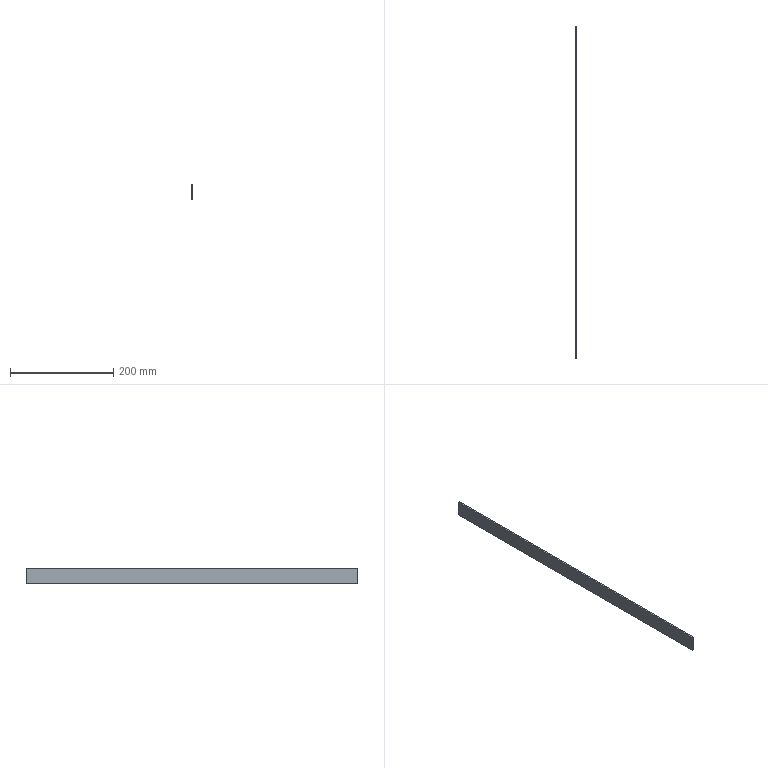Part | SolidWorks | 1 solid | 6 faces | box 3 x 642 x 30 mm | volume 57780 mm3 | plane 6
STEP:
#1=CARTESIAN_POINT('',(0.,321.,15.));
#2=VERTEX_POINT('',#1);
#3=CARTESIAN_POINT('',(0.,-321.,15.));
#4=VERTEX_POINT('',#3);
#5=CARTESIAN_POINT('',(0.,-321.,15.));
#6=DIRECTION('',(0.,-1.,0.));
#7=VECTOR('',#6,1000.);
#8=LINE('',#5,#7);
#9=EDGE_CURVE('',#2,#4,#8,.T.);
#10=ORIENTED_EDGE('',*,*,#9,.F.);
#11=CARTESIAN_POINT('',(-3.,321.,15.));
#12=VERTEX_POINT('',#11);
#13=CARTESIAN_POINT('',(-3.,321.,15.));
#14=DIRECTION('',(1.,0.,0.));
#15=VECTOR('',#14,1000.);
#16=LINE('',#13,#15);
#17=EDGE_CURVE('',#12,#2,#16,.T.);
#18=ORIENTED_EDGE('',*,*,#17,.F.);
#19=CARTESIAN_POINT('',(-3.,-321.,15.));
#20=VERTEX_POINT('',#19);
#21=CARTESIAN_POINT('',(-3.,-321.,15.));
#22=DIRECTION('',(0.,-1.,0.));
#23=VECTOR('',#22,1000.);
#24=LINE('',#21,#23);
#25=EDGE_CURVE('',#12,#20,#24,.T.);
#26=ORIENTED_EDGE('',*,*,#25,.T.);
#27=CARTESIAN_POINT('',(-3.,-321.,15.));
#28=DIRECTION('',(1.,0.,0.));
#29=VECTOR('',#28,1000.);
#30=LINE('',#27,#29);
#31=EDGE_CURVE('',#20,#4,#30,.T.);
#32=ORIENTED_EDGE('',*,*,#31,.T.);
#33=EDGE_LOOP('',(#10,#18,#26,#32));
#34=FACE_OUTER_BOUND('',#33,.T.);
#35=CARTESIAN_POINT('',(-3.,-321.,15.));
#36=DIRECTION('',(0.,0.,1.));
#37=DIRECTION('',(1.,0.,0.));
#38=AXIS2_PLACEMENT_3D('',#35,#36,#37);
#39=PLANE('',#38);
#40=ADVANCED_FACE('',(#34),#39,.T.);
#41=CARTESIAN_POINT('',(0.,321.,-15.));
#42=VERTEX_POINT('',#41);
#43=CARTESIAN_POINT('',(0.,321.,-15.));
#44=DIRECTION('',(0.,0.,1.));
#45=VECTOR('',#44,1000.);
#46=LINE('',#43,#45);
#47=EDGE_CURVE('',#42,#2,#46,.T.);
#48=ORIENTED_EDGE('',*,*,#47,.F.);
#49=CARTESIAN_POINT('',(-3.,321.,-15.));
#50=VERTEX_POINT('',#49);
#51=CARTESIAN_POINT('',(-3.,321.,-15.));
#52=DIRECTION('',(1.,0.,0.));
#53=VECTOR('',#52,1000.);
#54=LINE('',#51,#53);
#55=EDGE_CURVE('',#50,#42,#54,.T.);
#56=ORIENTED_EDGE('',*,*,#55,.F.);
#57=CARTESIAN_POINT('',(-3.,321.,-15.));
#58=DIRECTION('',(0.,0.,1.));
#59=VECTOR('',#58,1000.);
#60=LINE('',#57,#59);
#61=EDGE_CURVE('',#50,#12,#60,.T.);
#62=ORIENTED_EDGE('',*,*,#61,.T.);
#63=ORIENTED_EDGE('',*,*,#17,.T.);
#64=EDGE_LOOP('',(#48,#56,#62,#63));
#65=FACE_OUTER_BOUND('',#64,.T.);
#66=CARTESIAN_POINT('',(-3.,321.,-15.));
#67=DIRECTION('',(0.,1.,0.));
#68=DIRECTION('',(0.,0.,1.));
#69=AXIS2_PLACEMENT_3D('',#66,#67,#68);
#70=PLANE('',#69);
#71=ADVANCED_FACE('',(#65),#70,.T.);
#72=CARTESIAN_POINT('',(0.,-321.,-15.));
#73=VERTEX_POINT('',#72);
#74=CARTESIAN_POINT('',(0.,-321.,-15.));
#75=DIRECTION('',(0.,1.,0.));
#76=VECTOR('',#75,1000.);
#77=LINE('',#74,#76);
#78=EDGE_CURVE('',#73,#42,#77,.T.);
#79=ORIENTED_EDGE('',*,*,#78,.F.);
#80=CARTESIAN_POINT('',(-3.,-321.,-15.));
#81=VERTEX_POINT('',#80);
#82=CARTESIAN_POINT('',(-3.,-321.,-15.));
#83=DIRECTION('',(1.,0.,0.));
#84=VECTOR('',#83,1000.);
#85=LINE('',#82,#84);
#86=EDGE_CURVE('',#81,#73,#85,.T.);
#87=ORIENTED_EDGE('',*,*,#86,.F.);
#88=CARTESIAN_POINT('',(-3.,-321.,-15.));
#89=DIRECTION('',(0.,1.,0.));
#90=VECTOR('',#89,1000.);
#91=LINE('',#88,#90);
#92=EDGE_CURVE('',#81,#50,#91,.T.);
#93=ORIENTED_EDGE('',*,*,#92,.T.);
#94=ORIENTED_EDGE('',*,*,#55,.T.);
#95=EDGE_LOOP('',(#79,#87,#93,#94));
#96=FACE_OUTER_BOUND('',#95,.T.);
#97=CARTESIAN_POINT('',(-3.,-321.,-15.));
#98=DIRECTION('',(0.,0.,-1.));
#99=DIRECTION('',(0.,1.,0.));
#100=AXIS2_PLACEMENT_3D('',#97,#98,#99);
#101=PLANE('',#100);
#102=ADVANCED_FACE('',(#96),#101,.T.);
#103=CARTESIAN_POINT('',(0.,-321.,-15.));
#104=DIRECTION('',(0.,0.,-1.));
#105=VECTOR('',#104,1000.);
#106=LINE('',#103,#105);
#107=EDGE_CURVE('',#4,#73,#106,.T.);
#108=ORIENTED_EDGE('',*,*,#107,.F.);
#109=ORIENTED_EDGE('',*,*,#31,.F.);
#110=CARTESIAN_POINT('',(-3.,-321.,-15.));
#111=DIRECTION('',(0.,0.,-1.));
#112=VECTOR('',#111,1000.);
#113=LINE('',#110,#112);
#114=EDGE_CURVE('',#20,#81,#113,.T.);
#115=ORIENTED_EDGE('',*,*,#114,.T.);
#116=ORIENTED_EDGE('',*,*,#86,.T.);
#117=EDGE_LOOP('',(#108,#109,#115,#116));
#118=FACE_OUTER_BOUND('',#117,.T.);
#119=CARTESIAN_POINT('',(-3.,-321.,-15.));
#120=DIRECTION('',(0.,-1.,0.));
#121=DIRECTION('',(0.,0.,-1.));
#122=AXIS2_PLACEMENT_3D('',#119,#120,#121);
#123=PLANE('',#122);
#124=ADVANCED_FACE('',(#118),#123,.T.);
#125=ORIENTED_EDGE('',*,*,#25,.F.);
#126=ORIENTED_EDGE('',*,*,#61,.F.);
#127=ORIENTED_EDGE('',*,*,#92,.F.);
#128=ORIENTED_EDGE('',*,*,#114,.F.);
#129=EDGE_LOOP('',(#125,#126,#127,#128));
#130=FACE_OUTER_BOUND('',#129,.T.);
#131=CARTESIAN_POINT('',(-3.,0.,0.));
#132=DIRECTION('',(1.,0.,0.));
#133=DIRECTION('',(0.,0.,-1.));
#134=AXIS2_PLACEMENT_3D('',#131,#132,#133);
#135=PLANE('',#134);
#136=ADVANCED_FACE('',(#130),#135,.F.);
#137=ORIENTED_EDGE('',*,*,#9,.T.);
#138=ORIENTED_EDGE('',*,*,#107,.T.);
#139=ORIENTED_EDGE('',*,*,#78,.T.);
#140=ORIENTED_EDGE('',*,*,#47,.T.);
#141=EDGE_LOOP('',(#137,#138,#139,#140));
#142=FACE_OUTER_BOUND('',#141,.T.);
#143=CARTESIAN_POINT('',(0.,0.,0.));
#144=DIRECTION('',(1.,0.,0.));
#145=DIRECTION('',(0.,0.,-1.));
#146=AXIS2_PLACEMENT_3D('',#143,#144,#145);
#147=PLANE('',#146);
#148=ADVANCED_FACE('',(#142),#147,.T.);
#149=CLOSED_SHELL('',(#40,#71,#102,#124,#136,#148));
#150=MANIFOLD_SOLID_BREP('',#149);
#151=CARTESIAN_POINT('',(0.,0.,0.));
#152=DIRECTION('',(0.,0.,1.));
#153=DIRECTION('',(1.,0.,0.));
#154=AXIS2_PLACEMENT_3D('',#151,#152,#153);
#155=(LENGTH_UNIT()NAMED_UNIT(*)SI_UNIT(.MILLI.,.METRE.));
#156=UNCERTAINTY_MEASURE_WITH_UNIT(LENGTH_MEASURE(0.00001),#155,'','');
#157=(NAMED_UNIT(*)PLANE_ANGLE_UNIT()SI_UNIT($,.RADIAN.));
#158=(NAMED_UNIT(*)SI_UNIT($,.STERADIAN.)SOLID_ANGLE_UNIT());
#159=(GEOMETRIC_REPRESENTATION_CONTEXT(3)GLOBAL_UNCERTAINTY_ASSIGNED_CONTEXT((#156))GLOBAL_UNIT_ASSIGNED_CONTEXT((#155,#157,#158))REPRESENTATION_CONTEXT('',''));
#160=ADVANCED_BREP_SHAPE_REPRESENTATION('',(#150,#154),#159);